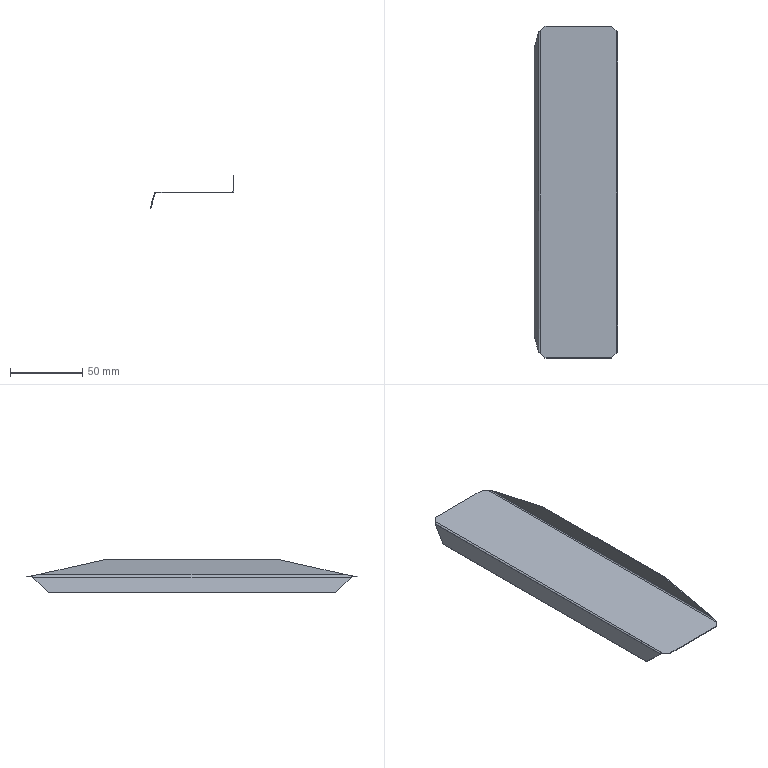Part | SolidWorks | features BaseBody 1 | 1 solid | 28 faces | box 57.977 x 230 x 22.893 mm | volume 8388 mm3 | plane 18 | spline 6 | cylinder 4 | commonest cylinder face diameters 1.5 x2 2.5 x2
STEP:
#1=CARTESIAN_POINT('',(-26.43,-111.57,0.));
#2=VERTEX_POINT('',#1);
#3=CARTESIAN_POINT('',(-26.43,111.57,0.));
#4=VERTEX_POINT('',#3);
#5=CARTESIAN_POINT('',(-26.43,0.,0.));
#6=DIRECTION('',(0.,1.,0.));
#7=VECTOR('',#6,1000.);
#8=LINE('',#5,#7);
#9=EDGE_CURVE('',#2,#4,#8,.T.);
#10=ORIENTED_EDGE('',*,*,#9,.F.);
#11=CARTESIAN_POINT('',(-23.,-115.,0.));
#12=VERTEX_POINT('',#11);
#13=CARTESIAN_POINT('',(-26.43,-111.57,0.));
#14=DIRECTION('',(-0.7071,0.7071,0.));
#15=VECTOR('',#14,1000.);
#16=LINE('',#13,#15);
#17=EDGE_CURVE('',#12,#2,#16,.T.);
#18=ORIENTED_EDGE('',*,*,#17,.F.);
#19=CARTESIAN_POINT('',(23.,-115.,0.));
#20=VERTEX_POINT('',#19);
#21=CARTESIAN_POINT('',(-0.1075,-115.,0.));
#22=DIRECTION('',(-1.,0.,0.));
#23=VECTOR('',#22,1000.);
#24=LINE('',#21,#23);
#25=EDGE_CURVE('',#20,#12,#24,.T.);
#26=ORIENTED_EDGE('',*,*,#25,.F.);
#27=CARTESIAN_POINT('',(26.215,-111.785,0.));
#28=VERTEX_POINT('',#27);
#29=CARTESIAN_POINT('',(23.,-115.,0.));
#30=DIRECTION('',(-0.7071,-0.7071,0.));
#31=VECTOR('',#30,1000.);
#32=LINE('',#29,#31);
#33=EDGE_CURVE('',#28,#20,#32,.T.);
#34=ORIENTED_EDGE('',*,*,#33,.F.);
#35=CARTESIAN_POINT('',(26.215,111.785,0.));
#36=VERTEX_POINT('',#35);
#37=CARTESIAN_POINT('',(26.215,0.,0.));
#38=DIRECTION('',(0.,-1.,0.));
#39=VECTOR('',#38,1000.);
#40=LINE('',#37,#39);
#41=EDGE_CURVE('',#36,#28,#40,.T.);
#42=ORIENTED_EDGE('',*,*,#41,.F.);
#43=CARTESIAN_POINT('',(23.,115.,0.));
#44=VERTEX_POINT('',#43);
#45=CARTESIAN_POINT('',(26.215,111.785,0.));
#46=DIRECTION('',(0.7071,-0.7071,0.));
#47=VECTOR('',#46,1000.);
#48=LINE('',#45,#47);
#49=EDGE_CURVE('',#44,#36,#48,.T.);
#50=ORIENTED_EDGE('',*,*,#49,.F.);
#51=CARTESIAN_POINT('',(-23.,115.,0.));
#52=VERTEX_POINT('',#51);
#53=CARTESIAN_POINT('',(-0.1075,115.,0.));
#54=DIRECTION('',(1.,0.,0.));
#55=VECTOR('',#54,1000.);
#56=LINE('',#53,#55);
#57=EDGE_CURVE('',#52,#44,#56,.T.);
#58=ORIENTED_EDGE('',*,*,#57,.F.);
#59=CARTESIAN_POINT('',(-23.,115.,0.));
#60=DIRECTION('',(0.7071,0.7071,0.));
#61=VECTOR('',#60,1000.);
#62=LINE('',#59,#61);
#63=EDGE_CURVE('',#4,#52,#62,.T.);
#64=ORIENTED_EDGE('',*,*,#63,.F.);
#65=EDGE_LOOP('',(#10,#18,#26,#34,#42,#50,#58,#64));
#66=FACE_OUTER_BOUND('',#65,.T.);
#67=CARTESIAN_POINT('',(26.215,-115.,0.));
#68=DIRECTION('',(0.,0.,-1.));
#69=DIRECTION('',(-1.,0.,0.));
#70=AXIS2_PLACEMENT_3D('',#67,#68,#69);
#71=PLANE('',#70);
#72=ADVANCED_FACE('',(#66),#71,.F.);
#73=CARTESIAN_POINT('',(-23.,115.,-0.5));
#74=VERTEX_POINT('',#73);
#75=CARTESIAN_POINT('',(-23.,115.,-0.25));
#76=DIRECTION('',(0.,0.,-1.));
#77=VECTOR('',#76,1000.);
#78=LINE('',#75,#77);
#79=EDGE_CURVE('',#52,#74,#78,.T.);
#80=ORIENTED_EDGE('',*,*,#79,.T.);
#81=CARTESIAN_POINT('',(-26.43,111.57,-0.5));
#82=VERTEX_POINT('',#81);
#83=CARTESIAN_POINT('',(-24.715,113.285,-0.5));
#84=DIRECTION('',(-0.7071,-0.7071,0.));
#85=VECTOR('',#84,1000.);
#86=LINE('',#83,#85);
#87=EDGE_CURVE('',#74,#82,#86,.T.);
#88=ORIENTED_EDGE('',*,*,#87,.T.);
#89=CARTESIAN_POINT('',(-26.43,111.57,-0.25));
#90=DIRECTION('',(0.,0.,1.));
#91=VECTOR('',#90,1000.);
#92=LINE('',#89,#91);
#93=EDGE_CURVE('',#82,#4,#92,.T.);
#94=ORIENTED_EDGE('',*,*,#93,.T.);
#95=ORIENTED_EDGE('',*,*,#63,.T.);
#96=EDGE_LOOP('',(#80,#88,#94,#95));
#97=FACE_OUTER_BOUND('',#96,.T.);
#98=CARTESIAN_POINT('',(-23.,115.,-0.5));
#99=DIRECTION('',(-0.7071,0.7071,0.));
#100=DIRECTION('',(-0.7071,-0.7071,0.));
#101=AXIS2_PLACEMENT_3D('',#98,#99,#100);
#102=PLANE('',#101);
#103=ADVANCED_FACE('',(#97),#102,.T.);
#104=CARTESIAN_POINT('',(-27.634,110.27,-0.916));
#105=VERTEX_POINT('',#104);
#106=CARTESIAN_POINT('',(-27.634,110.27,-0.916));
#107=CARTESIAN_POINT('',(-27.562,110.487,-0.6549));
#108=CARTESIAN_POINT('',(-27.402,110.703,-0.419));
#109=CARTESIAN_POINT('',(-26.971,111.137,-0.09103));
#110=CARTESIAN_POINT('',(-26.701,111.354,0.));
#111=CARTESIAN_POINT('',(-26.43,111.57,0.));
#112=B_SPLINE_CURVE_WITH_KNOTS('',3,(#106,#107,#108,#109,#110,#111),.UNSPECIFIED.,.F.,.F.,(4,2,4),(0.,0.5,1.),.UNSPECIFIED.);
#113=EDGE_CURVE('',#105,#4,#112,.T.);
#114=ORIENTED_EDGE('',*,*,#113,.F.);
#115=CARTESIAN_POINT('',(-27.634,-110.27,-0.916));
#116=VERTEX_POINT('',#115);
#117=CARTESIAN_POINT('',(-27.634,0.,-0.916));
#118=DIRECTION('',(0.,1.,0.));
#119=VECTOR('',#118,1000.);
#120=LINE('',#117,#119);
#121=EDGE_CURVE('',#116,#105,#120,.T.);
#122=ORIENTED_EDGE('',*,*,#121,.F.);
#123=CARTESIAN_POINT('',(-26.43,-111.57,0.));
#124=CARTESIAN_POINT('',(-26.701,-111.354,0.));
#125=CARTESIAN_POINT('',(-26.971,-111.137,-0.09103));
#126=CARTESIAN_POINT('',(-27.402,-110.703,-0.419));
#127=CARTESIAN_POINT('',(-27.562,-110.487,-0.6549));
#128=CARTESIAN_POINT('',(-27.634,-110.27,-0.916));
#129=B_SPLINE_CURVE_WITH_KNOTS('',3,(#123,#124,#125,#126,#127,#128),.UNSPECIFIED.,.F.,.F.,(4,2,4),(0.,0.5,1.),.UNSPECIFIED.);
#130=EDGE_CURVE('',#2,#116,#129,.T.);
#131=ORIENTED_EDGE('',*,*,#130,.F.);
#132=ORIENTED_EDGE('',*,*,#9,.T.);
#133=EDGE_LOOP('',(#114,#122,#131,#132));
#134=FACE_OUTER_BOUND('',#133,.T.);
#135=CARTESIAN_POINT('',(-26.43,-112.909,-1.25));
#136=DIRECTION('',(0.,1.,0.));
#137=DIRECTION('',(-1.,0.,0.));
#138=AXIS2_PLACEMENT_3D('',#135,#136,#137);
#139=CYLINDRICAL_SURFACE('',#138,1.25);
#140=ADVANCED_FACE('',(#134),#139,.T.);
#141=CARTESIAN_POINT('',(-23.,-115.,-0.5));
#142=VERTEX_POINT('',#141);
#143=CARTESIAN_POINT('',(-23.,-115.,-0.25));
#144=DIRECTION('',(0.,0.,1.));
#145=VECTOR('',#144,1000.);
#146=LINE('',#143,#145);
#147=EDGE_CURVE('',#142,#12,#146,.T.);
#148=ORIENTED_EDGE('',*,*,#147,.T.);
#149=ORIENTED_EDGE('',*,*,#17,.T.);
#150=CARTESIAN_POINT('',(-26.43,-111.57,-0.5));
#151=VERTEX_POINT('',#150);
#152=CARTESIAN_POINT('',(-26.43,-111.57,-0.25));
#153=DIRECTION('',(0.,0.,-1.));
#154=VECTOR('',#153,1000.);
#155=LINE('',#152,#154);
#156=EDGE_CURVE('',#2,#151,#155,.T.);
#157=ORIENTED_EDGE('',*,*,#156,.T.);
#158=CARTESIAN_POINT('',(-24.715,-113.285,-0.5));
#159=DIRECTION('',(0.7071,-0.7071,0.));
#160=VECTOR('',#159,1000.);
#161=LINE('',#158,#160);
#162=EDGE_CURVE('',#151,#142,#161,.T.);
#163=ORIENTED_EDGE('',*,*,#162,.T.);
#164=EDGE_LOOP('',(#148,#149,#157,#163));
#165=FACE_OUTER_BOUND('',#164,.T.);
#166=CARTESIAN_POINT('',(-26.43,-111.57,-0.5));
#167=DIRECTION('',(-0.7071,-0.7071,0.));
#168=DIRECTION('',(0.7071,-0.7071,0.));
#169=AXIS2_PLACEMENT_3D('',#166,#167,#168);
#170=PLANE('',#169);
#171=ADVANCED_FACE('',(#165),#170,.T.);
#172=CARTESIAN_POINT('',(23.,-115.,-0.5));
#173=VERTEX_POINT('',#172);
#174=CARTESIAN_POINT('',(0.,-115.,-0.5));
#175=DIRECTION('',(1.,0.,0.));
#176=VECTOR('',#175,1000.);
#177=LINE('',#174,#176);
#178=EDGE_CURVE('',#142,#173,#177,.T.);
#179=ORIENTED_EDGE('',*,*,#178,.T.);
#180=CARTESIAN_POINT('',(23.,-115.,-0.25));
#181=DIRECTION('',(0.,0.,1.));
#182=VECTOR('',#181,1000.);
#183=LINE('',#180,#182);
#184=EDGE_CURVE('',#173,#20,#183,.T.);
#185=ORIENTED_EDGE('',*,*,#184,.T.);
#186=ORIENTED_EDGE('',*,*,#25,.T.);
#187=ORIENTED_EDGE('',*,*,#147,.F.);
#188=EDGE_LOOP('',(#179,#185,#186,#187));
#189=FACE_OUTER_BOUND('',#188,.T.);
#190=CARTESIAN_POINT('',(-23.,-115.,-0.5));
#191=DIRECTION('',(0.,-1.,0.));
#192=DIRECTION('',(1.,0.,0.));
#193=AXIS2_PLACEMENT_3D('',#190,#191,#192);
#194=PLANE('',#193);
#195=ADVANCED_FACE('',(#189),#194,.T.);
#196=ORIENTED_EDGE('',*,*,#33,.T.);
#197=ORIENTED_EDGE('',*,*,#184,.F.);
#198=CARTESIAN_POINT('',(26.215,-111.785,-0.5));
#199=VERTEX_POINT('',#198);
#200=CARTESIAN_POINT('',(24.607,-113.393,-0.5));
#201=DIRECTION('',(0.7071,0.7071,0.));
#202=VECTOR('',#201,1000.);
#203=LINE('',#200,#202);
#204=EDGE_CURVE('',#173,#199,#203,.T.);
#205=ORIENTED_EDGE('',*,*,#204,.T.);
#206=CARTESIAN_POINT('',(26.215,-111.785,-0.25));
#207=DIRECTION('',(0.,0.,1.));
#208=VECTOR('',#207,1000.);
#209=LINE('',#206,#208);
#210=EDGE_CURVE('',#199,#28,#209,.T.);
#211=ORIENTED_EDGE('',*,*,#210,.T.);
#212=EDGE_LOOP('',(#196,#197,#205,#211));
#213=FACE_OUTER_BOUND('',#212,.T.);
#214=CARTESIAN_POINT('',(23.,-115.,-0.5));
#215=DIRECTION('',(0.7071,-0.7071,0.));
#216=DIRECTION('',(0.7071,0.7071,0.));
#217=AXIS2_PLACEMENT_3D('',#214,#215,#216);
#218=PLANE('',#217);
#219=ADVANCED_FACE('',(#213),#218,.T.);
#220=ORIENTED_EDGE('',*,*,#41,.T.);
#221=CARTESIAN_POINT('',(26.745,-111.,0.2197));
#222=VERTEX_POINT('',#221);
#223=CARTESIAN_POINT('',(26.215,-111.785,0.));
#224=CARTESIAN_POINT('',(26.411,-111.523,0.000000004));
#225=CARTESIAN_POINT('',(26.606,-111.262,0.08077));
#226=CARTESIAN_POINT('',(26.745,-111.,0.2197));
#227=B_SPLINE_CURVE_WITH_KNOTS('',3,(#223,#224,#225,#226),.UNSPECIFIED.,.F.,.F.,(4,4),(0.,0.0009817),.UNSPECIFIED.);
#228=EDGE_CURVE('',#28,#222,#227,.T.);
#229=ORIENTED_EDGE('',*,*,#228,.T.);
#230=CARTESIAN_POINT('',(26.965,-107.517,0.75));
#231=VERTEX_POINT('',#230);
#232=CARTESIAN_POINT('',(26.745,-111.,0.2197));
#233=CARTESIAN_POINT('',(26.884,-109.839,0.3585));
#234=CARTESIAN_POINT('',(26.965,-108.678,0.5536));
#235=CARTESIAN_POINT('',(26.965,-107.517,0.75));
#236=B_SPLINE_CURVE_WITH_KNOTS('',3,(#232,#233,#234,#235),.UNSPECIFIED.,.F.,.F.,(4,4),(0.,0.003533),.UNSPECIFIED.);
#237=EDGE_CURVE('',#222,#231,#236,.T.);
#238=ORIENTED_EDGE('',*,*,#237,.T.);
#239=CARTESIAN_POINT('',(26.965,107.517,0.75));
#240=VERTEX_POINT('',#239);
#241=CARTESIAN_POINT('',(26.965,0.,0.75));
#242=DIRECTION('',(0.,1.,0.));
#243=VECTOR('',#242,1000.);
#244=LINE('',#241,#243);
#245=EDGE_CURVE('',#231,#240,#244,.T.);
#246=ORIENTED_EDGE('',*,*,#245,.T.);
#247=CARTESIAN_POINT('',(26.745,111.,0.2197));
#248=VERTEX_POINT('',#247);
#249=CARTESIAN_POINT('',(26.965,107.517,0.75));
#250=CARTESIAN_POINT('',(26.965,108.678,0.5536));
#251=CARTESIAN_POINT('',(26.884,109.839,0.3585));
#252=CARTESIAN_POINT('',(26.745,111.,0.2197));
#253=B_SPLINE_CURVE_WITH_KNOTS('',3,(#249,#250,#251,#252),.UNSPECIFIED.,.F.,.F.,(4,4),(0.,0.003533),.UNSPECIFIED.);
#254=EDGE_CURVE('',#240,#248,#253,.T.);
#255=ORIENTED_EDGE('',*,*,#254,.T.);
#256=CARTESIAN_POINT('',(26.745,111.,0.2197));
#257=CARTESIAN_POINT('',(26.606,111.262,0.08073));
#258=CARTESIAN_POINT('',(26.411,111.523,0.000000004));
#259=CARTESIAN_POINT('',(26.215,111.785,0.));
#260=B_SPLINE_CURVE_WITH_KNOTS('',3,(#256,#257,#258,#259),.UNSPECIFIED.,.F.,.F.,(4,4),(0.,0.0009806),.UNSPECIFIED.);
#261=EDGE_CURVE('',#248,#36,#260,.T.);
#262=ORIENTED_EDGE('',*,*,#261,.T.);
#263=EDGE_LOOP('',(#220,#229,#238,#246,#255,#262));
#264=FACE_OUTER_BOUND('',#263,.T.);
#265=CARTESIAN_POINT('',(26.215,113.127,0.75));
#266=DIRECTION('',(0.,-1.,0.));
#267=DIRECTION('',(0.,0.,-1.));
#268=AXIS2_PLACEMENT_3D('',#265,#266,#267);
#269=CYLINDRICAL_SURFACE('',#268,0.75);
#270=ADVANCED_FACE('',(#264),#269,.F.);
#271=CARTESIAN_POINT('',(26.215,111.785,-0.5));
#272=VERTEX_POINT('',#271);
#273=CARTESIAN_POINT('',(23.,115.,-0.5));
#274=VERTEX_POINT('',#273);
#275=CARTESIAN_POINT('',(24.607,113.393,-0.5));
#276=DIRECTION('',(-0.7071,0.7071,0.));
#277=VECTOR('',#276,1000.);
#278=LINE('',#275,#277);
#279=EDGE_CURVE('',#272,#274,#278,.T.);
#280=ORIENTED_EDGE('',*,*,#279,.T.);
#281=CARTESIAN_POINT('',(23.,115.,-0.25));
#282=DIRECTION('',(0.,0.,1.));
#283=VECTOR('',#282,1000.);
#284=LINE('',#281,#283);
#285=EDGE_CURVE('',#274,#44,#284,.T.);
#286=ORIENTED_EDGE('',*,*,#285,.T.);
#287=ORIENTED_EDGE('',*,*,#49,.T.);
#288=CARTESIAN_POINT('',(26.215,111.785,-0.25));
#289=DIRECTION('',(0.,0.,-1.));
#290=VECTOR('',#289,1000.);
#291=LINE('',#288,#290);
#292=EDGE_CURVE('',#36,#272,#291,.T.);
#293=ORIENTED_EDGE('',*,*,#292,.T.);
#294=EDGE_LOOP('',(#280,#286,#287,#293));
#295=FACE_OUTER_BOUND('',#294,.T.);
#296=CARTESIAN_POINT('',(26.215,111.785,-0.5));
#297=DIRECTION('',(0.7071,0.7071,0.));
#298=DIRECTION('',(-0.7071,0.7071,0.));
#299=AXIS2_PLACEMENT_3D('',#296,#297,#298);
#300=PLANE('',#299);
#301=ADVANCED_FACE('',(#295),#300,.T.);
#302=CARTESIAN_POINT('',(0.,115.,-0.5));
#303=DIRECTION('',(-1.,0.,0.));
#304=VECTOR('',#303,1000.);
#305=LINE('',#302,#304);
#306=EDGE_CURVE('',#274,#74,#305,.T.);
#307=ORIENTED_EDGE('',*,*,#306,.T.);
#308=ORIENTED_EDGE('',*,*,#79,.F.);
#309=ORIENTED_EDGE('',*,*,#57,.T.);
#310=ORIENTED_EDGE('',*,*,#285,.F.);
#311=EDGE_LOOP('',(#307,#308,#309,#310));
#312=FACE_OUTER_BOUND('',#311,.T.);
#313=CARTESIAN_POINT('',(23.,115.,-0.5));
#314=DIRECTION('',(0.,1.,0.));
#315=DIRECTION('',(-1.,0.,0.));
#316=AXIS2_PLACEMENT_3D('',#313,#314,#315);
#317=PLANE('',#316);
#318=ADVANCED_FACE('',(#312),#317,.T.);
#319=ORIENTED_EDGE('',*,*,#178,.F.);
#320=ORIENTED_EDGE('',*,*,#162,.F.);
#321=CARTESIAN_POINT('',(-26.43,0.,-0.5));
#322=DIRECTION('',(0.,1.,0.));
#323=VECTOR('',#322,1000.);
#324=LINE('',#321,#323);
#325=EDGE_CURVE('',#151,#82,#324,.T.);
#326=ORIENTED_EDGE('',*,*,#325,.T.);
#327=ORIENTED_EDGE('',*,*,#87,.F.);
#328=ORIENTED_EDGE('',*,*,#306,.F.);
#329=ORIENTED_EDGE('',*,*,#279,.F.);
#330=CARTESIAN_POINT('',(26.215,0.,-0.5));
#331=DIRECTION('',(0.,-1.,0.));
#332=VECTOR('',#331,1000.);
#333=LINE('',#330,#332);
#334=EDGE_CURVE('',#272,#199,#333,.T.);
#335=ORIENTED_EDGE('',*,*,#334,.T.);
#336=ORIENTED_EDGE('',*,*,#204,.F.);
#337=EDGE_LOOP('',(#319,#320,#326,#327,#328,#329,#335,#336));
#338=FACE_OUTER_BOUND('',#337,.T.);
#339=CARTESIAN_POINT('',(26.215,-115.,-0.5));
#340=DIRECTION('',(0.,0.,-1.));
#341=DIRECTION('',(-1.,0.,0.));
#342=AXIS2_PLACEMENT_3D('',#339,#340,#341);
#343=PLANE('',#342);
#344=ADVANCED_FACE('',(#338),#343,.T.);
#345=ORIENTED_EDGE('',*,*,#113,.T.);
#346=ORIENTED_EDGE('',*,*,#93,.F.);
#347=CARTESIAN_POINT('',(-27.152,110.27,-1.05));
#348=VERTEX_POINT('',#347);
#349=CARTESIAN_POINT('',(-27.152,110.27,-1.05));
#350=CARTESIAN_POINT('',(-27.109,110.487,-0.8929));
#351=CARTESIAN_POINT('',(-27.013,110.703,-0.7514));
#352=CARTESIAN_POINT('',(-26.754,111.137,-0.5546));
#353=CARTESIAN_POINT('',(-26.592,111.354,-0.5));
#354=CARTESIAN_POINT('',(-26.43,111.57,-0.5));
#355=B_SPLINE_CURVE_WITH_KNOTS('',3,(#349,#350,#351,#352,#353,#354),.UNSPECIFIED.,.F.,.F.,(4,2,4),(0.,0.5,1.),.UNSPECIFIED.);
#356=EDGE_CURVE('',#348,#82,#355,.T.);
#357=ORIENTED_EDGE('',*,*,#356,.F.);
#358=CARTESIAN_POINT('',(-27.393,110.27,-0.9828));
#359=DIRECTION('',(0.9636,0.,-0.2672));
#360=VECTOR('',#359,1000.);
#361=LINE('',#358,#360);
#362=EDGE_CURVE('',#105,#348,#361,.T.);
#363=ORIENTED_EDGE('',*,*,#362,.F.);
#364=EDGE_LOOP('',(#345,#346,#357,#363));
#365=FACE_OUTER_BOUND('',#364,.T.);
#366=CARTESIAN_POINT('',(-27.639,110.27,-0.9146));
#367=CARTESIAN_POINT('',(-27.603,110.378,-0.7836));
#368=CARTESIAN_POINT('',(-27.545,110.487,-0.6585));
#369=CARTESIAN_POINT('',(-27.392,110.703,-0.4334));
#370=CARTESIAN_POINT('',(-27.298,110.812,-0.3333));
#371=CARTESIAN_POINT('',(-27.081,111.029,-0.1687));
#372=CARTESIAN_POINT('',(-26.959,111.137,-0.1042));
#373=CARTESIAN_POINT('',(-26.702,111.354,-0.01729));
#374=CARTESIAN_POINT('',(-26.566,111.462,0.005));
#375=CARTESIAN_POINT('',(-26.43,111.57,0.005));
#376=CARTESIAN_POINT('',(-27.634,110.27,-0.916));
#377=CARTESIAN_POINT('',(-27.598,110.378,-0.7854));
#378=CARTESIAN_POINT('',(-27.54,110.487,-0.6609));
#379=CARTESIAN_POINT('',(-27.388,110.703,-0.4366));
#380=CARTESIAN_POINT('',(-27.294,110.812,-0.337));
#381=CARTESIAN_POINT('',(-27.078,111.029,-0.173));
#382=CARTESIAN_POINT('',(-26.957,111.137,-0.1087));
#383=CARTESIAN_POINT('',(-26.701,111.354,-0.02221));
#384=CARTESIAN_POINT('',(-26.565,111.462,0.));
#385=CARTESIAN_POINT('',(-26.43,111.57,0.));
#386=CARTESIAN_POINT('',(-27.152,110.27,-1.05));
#387=CARTESIAN_POINT('',(-27.131,110.378,-0.9713));
#388=CARTESIAN_POINT('',(-27.096,110.487,-0.8965));
#389=CARTESIAN_POINT('',(-27.005,110.703,-0.762));
#390=CARTESIAN_POINT('',(-26.948,110.812,-0.7022));
#391=CARTESIAN_POINT('',(-26.819,111.029,-0.6038));
#392=CARTESIAN_POINT('',(-26.746,111.137,-0.5652));
#393=CARTESIAN_POINT('',(-26.592,111.354,-0.5133));
#394=CARTESIAN_POINT('',(-26.511,111.462,-0.5));
#395=CARTESIAN_POINT('',(-26.43,111.57,-0.5));
#396=CARTESIAN_POINT('',(-27.148,110.27,-1.051));
#397=CARTESIAN_POINT('',(-27.126,110.378,-0.9731));
#398=CARTESIAN_POINT('',(-27.092,110.487,-0.8989));
#399=CARTESIAN_POINT('',(-27.001,110.703,-0.7653));
#400=CARTESIAN_POINT('',(-26.945,110.812,-0.7059));
#401=CARTESIAN_POINT('',(-26.816,111.029,-0.6082));
#402=CARTESIAN_POINT('',(-26.744,111.137,-0.5698));
#403=CARTESIAN_POINT('',(-26.591,111.354,-0.5183));
#404=CARTESIAN_POINT('',(-26.51,111.462,-0.505));
#405=CARTESIAN_POINT('',(-26.43,111.57,-0.505));
#406=B_SPLINE_SURFACE_WITH_KNOTS('',1,3,((#366,#367,#368,#369,#370,#371,#372,#373,#374,#375),(#376,#377,#378,#379,#380,#381,#382,#383,#384,#385),(#386,#387,#388,#389,#390,#391,#392,#393,#394,#395),(#396,#397,#398,#399,#400,#401,#402,#403,#404,#405)),.UNSPECIFIED.,.F.,.F.,.F.,(2,1,1,2),(4,2,2,2,4),(-0.01,0.,1.,1.01),(0.,0.25,0.5,0.75,1.),.UNSPECIFIED.);
#407=ADVANCED_FACE('',(#365),#406,.F.);
#408=CARTESIAN_POINT('',(-30.512,99.5,-11.294));
#409=VERTEX_POINT('',#408);
#410=CARTESIAN_POINT('',(-27.634,110.27,-0.916));
#411=DIRECTION('',(0.189,0.7071,0.6814));
#412=VECTOR('',#411,1000.);
#413=LINE('',#410,#412);
#414=EDGE_CURVE('',#409,#105,#413,.T.);
#415=ORIENTED_EDGE('',*,*,#414,.F.);
#416=CARTESIAN_POINT('',(-30.512,-99.5,-11.294));
#417=VERTEX_POINT('',#416);
#418=CARTESIAN_POINT('',(-30.512,0.,-11.294));
#419=DIRECTION('',(0.,1.,0.));
#420=VECTOR('',#419,1000.);
#421=LINE('',#418,#420);
#422=EDGE_CURVE('',#417,#409,#421,.T.);
#423=ORIENTED_EDGE('',*,*,#422,.F.);
#424=CARTESIAN_POINT('',(-30.512,-99.5,-11.294));
#425=DIRECTION('',(-0.189,0.7071,-0.6814));
#426=VECTOR('',#425,1000.);
#427=LINE('',#424,#426);
#428=EDGE_CURVE('',#116,#417,#427,.T.);
#429=ORIENTED_EDGE('',*,*,#428,.F.);
#430=ORIENTED_EDGE('',*,*,#121,.T.);
#431=EDGE_LOOP('',(#415,#423,#429,#430));
#432=FACE_OUTER_BOUND('',#431,.T.);
#433=CARTESIAN_POINT('',(-27.634,-111.593,-0.916));
#434=DIRECTION('',(0.9636,0.,-0.2672));
#435=DIRECTION('',(-0.2672,0.,-0.9636));
#436=AXIS2_PLACEMENT_3D('',#433,#434,#435);
#437=PLANE('',#436);
#438=ADVANCED_FACE('',(#432),#437,.F.);
#439=CARTESIAN_POINT('',(-27.152,-110.27,-1.05));
#440=VERTEX_POINT('',#439);
#441=CARTESIAN_POINT('',(-27.393,-110.27,-0.9828));
#442=DIRECTION('',(-0.9636,0.,0.2672));
#443=VECTOR('',#442,1000.);
#444=LINE('',#441,#443);
#445=EDGE_CURVE('',#440,#116,#444,.T.);
#446=ORIENTED_EDGE('',*,*,#445,.F.);
#447=CARTESIAN_POINT('',(-26.43,-111.57,-0.5));
#448=CARTESIAN_POINT('',(-26.592,-111.354,-0.5));
#449=CARTESIAN_POINT('',(-26.754,-111.137,-0.5546));
#450=CARTESIAN_POINT('',(-27.013,-110.703,-0.7514));
#451=CARTESIAN_POINT('',(-27.109,-110.487,-0.8929));
#452=CARTESIAN_POINT('',(-27.152,-110.27,-1.05));
#453=B_SPLINE_CURVE_WITH_KNOTS('',3,(#447,#448,#449,#450,#451,#452),.UNSPECIFIED.,.F.,.F.,(4,2,4),(0.,0.5,1.),.UNSPECIFIED.);
#454=EDGE_CURVE('',#151,#440,#453,.T.);
#455=ORIENTED_EDGE('',*,*,#454,.F.);
#456=ORIENTED_EDGE('',*,*,#156,.F.);
#457=ORIENTED_EDGE('',*,*,#130,.T.);
#458=EDGE_LOOP('',(#446,#455,#456,#457));
#459=FACE_OUTER_BOUND('',#458,.T.);
#460=CARTESIAN_POINT('',(-26.43,-111.57,0.005));
#461=CARTESIAN_POINT('',(-26.566,-111.462,0.005));
#462=CARTESIAN_POINT('',(-26.702,-111.354,-0.01729));
#463=CARTESIAN_POINT('',(-26.959,-111.137,-0.1042));
#464=CARTESIAN_POINT('',(-27.081,-111.029,-0.1687));
#465=CARTESIAN_POINT('',(-27.298,-110.812,-0.3333));
#466=CARTESIAN_POINT('',(-27.392,-110.703,-0.4334));
#467=CARTESIAN_POINT('',(-27.545,-110.487,-0.6585));
#468=CARTESIAN_POINT('',(-27.603,-110.378,-0.7836));
#469=CARTESIAN_POINT('',(-27.639,-110.27,-0.9146));
#470=CARTESIAN_POINT('',(-26.43,-111.57,0.));
#471=CARTESIAN_POINT('',(-26.565,-111.462,0.));
#472=CARTESIAN_POINT('',(-26.701,-111.354,-0.02221));
#473=CARTESIAN_POINT('',(-26.957,-111.137,-0.1087));
#474=CARTESIAN_POINT('',(-27.078,-111.029,-0.173));
#475=CARTESIAN_POINT('',(-27.294,-110.812,-0.337));
#476=CARTESIAN_POINT('',(-27.388,-110.703,-0.4366));
#477=CARTESIAN_POINT('',(-27.54,-110.487,-0.6609));
#478=CARTESIAN_POINT('',(-27.598,-110.378,-0.7854));
#479=CARTESIAN_POINT('',(-27.634,-110.27,-0.916));
#480=CARTESIAN_POINT('',(-26.43,-111.57,-0.5));
#481=CARTESIAN_POINT('',(-26.511,-111.462,-0.5));
#482=CARTESIAN_POINT('',(-26.592,-111.354,-0.5133));
#483=CARTESIAN_POINT('',(-26.746,-111.137,-0.5652));
#484=CARTESIAN_POINT('',(-26.819,-111.029,-0.6038));
#485=CARTESIAN_POINT('',(-26.948,-110.812,-0.7022));
#486=CARTESIAN_POINT('',(-27.005,-110.703,-0.762));
#487=CARTESIAN_POINT('',(-27.096,-110.487,-0.8965));
#488=CARTESIAN_POINT('',(-27.131,-110.378,-0.9713));
#489=CARTESIAN_POINT('',(-27.152,-110.27,-1.05));
#490=CARTESIAN_POINT('',(-26.43,-111.57,-0.505));
#491=CARTESIAN_POINT('',(-26.51,-111.462,-0.505));
#492=CARTESIAN_POINT('',(-26.591,-111.354,-0.5183));
#493=CARTESIAN_POINT('',(-26.744,-111.137,-0.5698));
#494=CARTESIAN_POINT('',(-26.816,-111.029,-0.6082));
#495=CARTESIAN_POINT('',(-26.945,-110.812,-0.7059));
#496=CARTESIAN_POINT('',(-27.001,-110.703,-0.7653));
#497=CARTESIAN_POINT('',(-27.092,-110.487,-0.8989));
#498=CARTESIAN_POINT('',(-27.126,-110.378,-0.9731));
#499=CARTESIAN_POINT('',(-27.148,-110.27,-1.051));
#500=B_SPLINE_SURFACE_WITH_KNOTS('',1,3,((#460,#461,#462,#463,#464,#465,#466,#467,#468,#469),(#470,#471,#472,#473,#474,#475,#476,#477,#478,#479),(#480,#481,#482,#483,#484,#485,#486,#487,#488,#489),(#490,#491,#492,#493,#494,#495,#496,#497,#498,#499)),.UNSPECIFIED.,.F.,.F.,.F.,(2,1,1,2),(4,2,2,2,4),(-0.01,0.,1.,1.01),(0.,0.25,0.5,0.75,1.),.UNSPECIFIED.);
#501=ADVANCED_FACE('',(#459),#500,.F.);
#502=CARTESIAN_POINT('',(27.098,-111.,-0.1339));
#503=VERTEX_POINT('',#502);
#504=CARTESIAN_POINT('',(26.215,-111.785,-0.5));
#505=CARTESIAN_POINT('',(26.379,-111.654,-0.5));
#506=CARTESIAN_POINT('',(26.542,-111.523,-0.4674));
#507=CARTESIAN_POINT('',(26.845,-111.261,-0.3416));
#508=CARTESIAN_POINT('',(26.982,-111.131,-0.2501));
#509=CARTESIAN_POINT('',(27.098,-111.,-0.1339));
#510=B_SPLINE_CURVE_WITH_KNOTS('',3,(#504,#505,#506,#507,#508,#509),.UNSPECIFIED.,.F.,.F.,(4,2,4),(0.,0.0006291,0.001258),.UNSPECIFIED.);
#511=EDGE_CURVE('',#199,#503,#510,.T.);
#512=ORIENTED_EDGE('',*,*,#511,.T.);
#513=CARTESIAN_POINT('',(26.922,-111.,0.04289));
#514=DIRECTION('',(-0.7071,0.,0.7071));
#515=VECTOR('',#514,1000.);
#516=LINE('',#513,#515);
#517=EDGE_CURVE('',#503,#222,#516,.T.);
#518=ORIENTED_EDGE('',*,*,#517,.T.);
#519=ORIENTED_EDGE('',*,*,#228,.F.);
#520=ORIENTED_EDGE('',*,*,#210,.F.);
#521=EDGE_LOOP('',(#512,#518,#519,#520));
#522=FACE_OUTER_BOUND('',#521,.T.);
#523=CARTESIAN_POINT('',(27.102,-111.,-0.1375));
#524=CARTESIAN_POINT('',(26.986,-111.131,-0.2536));
#525=CARTESIAN_POINT('',(26.847,-111.262,-0.3466));
#526=CARTESIAN_POINT('',(26.543,-111.524,-0.4724));
#527=CARTESIAN_POINT('',(26.379,-111.654,-0.505));
#528=CARTESIAN_POINT('',(26.215,-111.785,-0.505));
#529=CARTESIAN_POINT('',(27.098,-111.,-0.1339));
#530=CARTESIAN_POINT('',(26.983,-111.131,-0.2496));
#531=CARTESIAN_POINT('',(26.844,-111.262,-0.3422));
#532=CARTESIAN_POINT('',(26.542,-111.524,-0.4675));
#533=CARTESIAN_POINT('',(26.378,-111.654,-0.5));
#534=CARTESIAN_POINT('',(26.215,-111.785,-0.5));
#535=CARTESIAN_POINT('',(26.745,-111.,0.2197));
#536=CARTESIAN_POINT('',(26.676,-111.131,0.1502));
#537=CARTESIAN_POINT('',(26.592,-111.262,0.09466));
#538=CARTESIAN_POINT('',(26.411,-111.524,0.01952));
#539=CARTESIAN_POINT('',(26.313,-111.654,0.));
#540=CARTESIAN_POINT('',(26.215,-111.785,0.));
#541=CARTESIAN_POINT('',(26.741,-111.,0.2232));
#542=CARTESIAN_POINT('',(26.672,-111.131,0.1542));
#543=CARTESIAN_POINT('',(26.59,-111.262,0.09903));
#544=CARTESIAN_POINT('',(26.41,-111.524,0.02439));
#545=CARTESIAN_POINT('',(26.312,-111.654,0.005));
#546=CARTESIAN_POINT('',(26.215,-111.785,0.005));
#547=B_SPLINE_SURFACE_WITH_KNOTS('',1,3,((#523,#524,#525,#526,#527,#528),(#529,#530,#531,#532,#533,#534),(#535,#536,#537,#538,#539,#540),(#541,#542,#543,#544,#545,#546)),.UNSPECIFIED.,.F.,.F.,.F.,(2,1,1,2),(4,2,4),(-0.0101,0.,1.,1.01),(0.,0.5,1.),.UNSPECIFIED.);
#548=ADVANCED_FACE('',(#522),#547,.T.);
#549=CARTESIAN_POINT('',(27.098,111.,-0.1339));
#550=VERTEX_POINT('',#549);
#551=CARTESIAN_POINT('',(26.922,111.,0.04289));
#552=DIRECTION('',(0.7071,0.,-0.7071));
#553=VECTOR('',#552,1000.);
#554=LINE('',#551,#553);
#555=EDGE_CURVE('',#248,#550,#554,.T.);
#556=ORIENTED_EDGE('',*,*,#555,.T.);
#557=CARTESIAN_POINT('',(27.098,111.,-0.1339));
#558=CARTESIAN_POINT('',(26.982,111.131,-0.2501));
#559=CARTESIAN_POINT('',(26.844,111.262,-0.3425));
#560=CARTESIAN_POINT('',(26.541,111.525,-0.4679));
#561=CARTESIAN_POINT('',(26.379,111.654,-0.5));
#562=CARTESIAN_POINT('',(26.215,111.785,-0.5));
#563=B_SPLINE_CURVE_WITH_KNOTS('',3,(#557,#558,#559,#560,#561,#562),.UNSPECIFIED.,.F.,.F.,(4,2,4),(0.,0.0006291,0.001258),.UNSPECIFIED.);
#564=EDGE_CURVE('',#550,#272,#563,.T.);
#565=ORIENTED_EDGE('',*,*,#564,.T.);
#566=ORIENTED_EDGE('',*,*,#292,.F.);
#567=ORIENTED_EDGE('',*,*,#261,.F.);
#568=EDGE_LOOP('',(#556,#565,#566,#567));
#569=FACE_OUTER_BOUND('',#568,.T.);
#570=CARTESIAN_POINT('',(26.215,111.785,-0.505));
#571=CARTESIAN_POINT('',(26.379,111.654,-0.505));
#572=CARTESIAN_POINT('',(26.543,111.524,-0.4724));
#573=CARTESIAN_POINT('',(26.847,111.262,-0.3466));
#574=CARTESIAN_POINT('',(26.986,111.131,-0.2536));
#575=CARTESIAN_POINT('',(27.102,111.,-0.1375));
#576=CARTESIAN_POINT('',(27.104,110.997,-0.1351));
#577=CARTESIAN_POINT('',(27.107,110.995,-0.1328));
#578=CARTESIAN_POINT('',(27.109,110.992,-0.1305));
#579=CARTESIAN_POINT('',(26.215,111.785,-0.5));
#580=CARTESIAN_POINT('',(26.378,111.654,-0.5));
#581=CARTESIAN_POINT('',(26.542,111.524,-0.4675));
#582=CARTESIAN_POINT('',(26.844,111.262,-0.3422));
#583=CARTESIAN_POINT('',(26.983,111.131,-0.2496));
#584=CARTESIAN_POINT('',(27.098,111.,-0.1339));
#585=CARTESIAN_POINT('',(27.101,110.997,-0.1316));
#586=CARTESIAN_POINT('',(27.103,110.995,-0.1293));
#587=CARTESIAN_POINT('',(27.105,110.992,-0.1269));
#588=CARTESIAN_POINT('',(26.215,111.785,0.));
#589=CARTESIAN_POINT('',(26.313,111.654,0.));
#590=CARTESIAN_POINT('',(26.411,111.524,0.01952));
#591=CARTESIAN_POINT('',(26.592,111.262,0.09466));
#592=CARTESIAN_POINT('',(26.676,111.131,0.1502));
#593=CARTESIAN_POINT('',(26.745,111.,0.2197));
#594=CARTESIAN_POINT('',(26.746,110.997,0.2211));
#595=CARTESIAN_POINT('',(26.748,110.995,0.2224));
#596=CARTESIAN_POINT('',(26.749,110.992,0.2238));
#597=CARTESIAN_POINT('',(26.215,111.785,0.005));
#598=CARTESIAN_POINT('',(26.312,111.654,0.005));
#599=CARTESIAN_POINT('',(26.41,111.524,0.02439));
#600=CARTESIAN_POINT('',(26.59,111.262,0.09903));
#601=CARTESIAN_POINT('',(26.672,111.131,0.1542));
#602=CARTESIAN_POINT('',(26.741,111.,0.2232));
#603=CARTESIAN_POINT('',(26.743,110.997,0.2246));
#604=CARTESIAN_POINT('',(26.744,110.995,0.226));
#605=CARTESIAN_POINT('',(26.746,110.992,0.2273));
#606=B_SPLINE_SURFACE_WITH_KNOTS('',1,3,((#570,#571,#572,#573,#574,#575,#576,#577,#578),(#579,#580,#581,#582,#583,#584,#585,#586,#587),(#588,#589,#590,#591,#592,#593,#594,#595,#596),(#597,#598,#599,#600,#601,#602,#603,#604,#605)),.UNSPECIFIED.,.F.,.F.,.F.,(2,1,1,2),(4,2,3,4),(-0.0101,0.,1.,1.01),(0.,0.5,1.,1.01),.UNSPECIFIED.);
#607=ADVANCED_FACE('',(#569),#606,.T.);
#608=CARTESIAN_POINT('',(27.465,107.517,0.75));
#609=VERTEX_POINT('',#608);
#610=CARTESIAN_POINT('',(27.215,107.517,0.75));
#611=DIRECTION('',(-1.,0.,0.));
#612=VECTOR('',#611,1000.);
#613=LINE('',#610,#612);
#614=EDGE_CURVE('',#609,#240,#613,.T.);
#615=ORIENTED_EDGE('',*,*,#614,.F.);
#616=CARTESIAN_POINT('',(27.465,107.517,0.75));
#617=CARTESIAN_POINT('',(27.465,108.098,0.5863));
#618=CARTESIAN_POINT('',(27.432,108.678,0.4228));
#619=CARTESIAN_POINT('',(27.307,109.839,0.1204));
#620=CARTESIAN_POINT('',(27.214,110.419,-0.01813));
#621=CARTESIAN_POINT('',(27.098,111.,-0.1339));
#622=B_SPLINE_CURVE_WITH_KNOTS('',3,(#616,#617,#618,#619,#620,#621),.UNSPECIFIED.,.F.,.F.,(4,2,4),(0.,0.001809,0.003619),.UNSPECIFIED.);
#623=EDGE_CURVE('',#609,#550,#622,.T.);
#624=ORIENTED_EDGE('',*,*,#623,.T.);
#625=ORIENTED_EDGE('',*,*,#555,.F.);
#626=ORIENTED_EDGE('',*,*,#254,.F.);
#627=EDGE_LOOP('',(#615,#624,#625,#626));
#628=FACE_OUTER_BOUND('',#627,.T.);
#629=CARTESIAN_POINT('',(27.102,111.,-0.1375));
#630=CARTESIAN_POINT('',(27.218,110.419,-0.02129));
#631=CARTESIAN_POINT('',(27.311,109.839,0.1179));
#632=CARTESIAN_POINT('',(27.437,108.678,0.4215));
#633=CARTESIAN_POINT('',(27.47,108.097,0.5857));
#634=CARTESIAN_POINT('',(27.47,107.517,0.75));
#635=CARTESIAN_POINT('',(27.098,111.,-0.1339));
#636=CARTESIAN_POINT('',(27.214,110.419,-0.01818));
#637=CARTESIAN_POINT('',(27.307,109.839,0.1205));
#638=CARTESIAN_POINT('',(27.432,108.678,0.4228));
#639=CARTESIAN_POINT('',(27.465,108.097,0.5864));
#640=CARTESIAN_POINT('',(27.465,107.517,0.75));
#641=CARTESIAN_POINT('',(26.745,111.,0.2197));
#642=CARTESIAN_POINT('',(26.814,110.419,0.2891));
#643=CARTESIAN_POINT('',(26.87,109.839,0.3723));
#644=CARTESIAN_POINT('',(26.945,108.678,0.5537));
#645=CARTESIAN_POINT('',(26.965,108.097,0.6518));
#646=CARTESIAN_POINT('',(26.965,107.517,0.75));
#647=CARTESIAN_POINT('',(26.741,111.,0.2232));
#648=CARTESIAN_POINT('',(26.81,110.419,0.2922));
#649=CARTESIAN_POINT('',(26.866,109.839,0.3748));
#650=CARTESIAN_POINT('',(26.94,108.678,0.555));
#651=CARTESIAN_POINT('',(26.96,108.097,0.6525));
#652=CARTESIAN_POINT('',(26.96,107.517,0.75));
#653=B_SPLINE_SURFACE_WITH_KNOTS('',1,3,((#629,#630,#631,#632,#633,#634),(#635,#636,#637,#638,#639,#640),(#641,#642,#643,#644,#645,#646),(#647,#648,#649,#650,#651,#652)),.UNSPECIFIED.,.F.,.F.,.F.,(2,1,1,2),(4,2,4),(-0.0101,0.,1.,1.01),(0.,0.5,1.),.UNSPECIFIED.);
#654=ADVANCED_FACE('',(#628),#653,.T.);
#655=ORIENTED_EDGE('',*,*,#245,.F.);
#656=CARTESIAN_POINT('',(26.965,-60.,11.465));
#657=VERTEX_POINT('',#656);
#658=CARTESIAN_POINT('',(26.965,-107.517,0.75));
#659=DIRECTION('',(0.,-0.9755,-0.22));
#660=VECTOR('',#659,1000.);
#661=LINE('',#658,#660);
#662=EDGE_CURVE('',#657,#231,#661,.T.);
#663=ORIENTED_EDGE('',*,*,#662,.F.);
#664=CARTESIAN_POINT('',(26.965,60.,11.465));
#665=VERTEX_POINT('',#664);
#666=CARTESIAN_POINT('',(26.965,0.,11.465));
#667=DIRECTION('',(0.,-1.,0.));
#668=VECTOR('',#667,1000.);
#669=LINE('',#666,#668);
#670=EDGE_CURVE('',#665,#657,#669,.T.);
#671=ORIENTED_EDGE('',*,*,#670,.F.);
#672=CARTESIAN_POINT('',(26.965,60.,11.465));
#673=DIRECTION('',(0.,-0.9755,0.22));
#674=VECTOR('',#673,1000.);
#675=LINE('',#672,#674);
#676=EDGE_CURVE('',#240,#665,#675,.T.);
#677=ORIENTED_EDGE('',*,*,#676,.F.);
#678=EDGE_LOOP('',(#655,#663,#671,#677));
#679=FACE_OUTER_BOUND('',#678,.T.);
#680=CARTESIAN_POINT('',(26.965,-108.807,11.465));
#681=DIRECTION('',(1.,0.,0.));
#682=DIRECTION('',(0.,0.,-1.));
#683=AXIS2_PLACEMENT_3D('',#680,#681,#682);
#684=PLANE('',#683);
#685=ADVANCED_FACE('',(#679),#684,.F.);
#686=ORIENTED_EDGE('',*,*,#517,.F.);
#687=CARTESIAN_POINT('',(27.465,-107.517,0.75));
#688=VERTEX_POINT('',#687);
#689=CARTESIAN_POINT('',(27.098,-111.,-0.1339));
#690=CARTESIAN_POINT('',(27.214,-110.419,-0.01813));
#691=CARTESIAN_POINT('',(27.307,-109.839,0.1205));
#692=CARTESIAN_POINT('',(27.432,-108.678,0.4229));
#693=CARTESIAN_POINT('',(27.465,-108.098,0.5863));
#694=CARTESIAN_POINT('',(27.465,-107.517,0.75));
#695=B_SPLINE_CURVE_WITH_KNOTS('',3,(#689,#690,#691,#692,#693,#694),.UNSPECIFIED.,.F.,.F.,(4,2,4),(0.,0.001809,0.003619),.UNSPECIFIED.);
#696=EDGE_CURVE('',#503,#688,#695,.T.);
#697=ORIENTED_EDGE('',*,*,#696,.T.);
#698=CARTESIAN_POINT('',(27.215,-107.517,0.75));
#699=DIRECTION('',(-1.,0.,0.));
#700=VECTOR('',#699,1000.);
#701=LINE('',#698,#700);
#702=EDGE_CURVE('',#688,#231,#701,.T.);
#703=ORIENTED_EDGE('',*,*,#702,.T.);
#704=ORIENTED_EDGE('',*,*,#237,.F.);
#705=EDGE_LOOP('',(#686,#697,#703,#704));
#706=FACE_OUTER_BOUND('',#705,.T.);
#707=CARTESIAN_POINT('',(27.47,-107.517,0.75));
#708=CARTESIAN_POINT('',(27.47,-108.097,0.5857));
#709=CARTESIAN_POINT('',(27.437,-108.678,0.4215));
#710=CARTESIAN_POINT('',(27.311,-109.839,0.1179));
#711=CARTESIAN_POINT('',(27.218,-110.419,-0.02129));
#712=CARTESIAN_POINT('',(27.102,-111.,-0.1375));
#713=CARTESIAN_POINT('',(27.465,-107.517,0.75));
#714=CARTESIAN_POINT('',(27.465,-108.097,0.5864));
#715=CARTESIAN_POINT('',(27.432,-108.678,0.4228));
#716=CARTESIAN_POINT('',(27.307,-109.839,0.1205));
#717=CARTESIAN_POINT('',(27.214,-110.419,-0.01818));
#718=CARTESIAN_POINT('',(27.098,-111.,-0.1339));
#719=CARTESIAN_POINT('',(26.965,-107.517,0.75));
#720=CARTESIAN_POINT('',(26.965,-108.097,0.6518));
#721=CARTESIAN_POINT('',(26.945,-108.678,0.5537));
#722=CARTESIAN_POINT('',(26.87,-109.839,0.3723));
#723=CARTESIAN_POINT('',(26.814,-110.419,0.2891));
#724=CARTESIAN_POINT('',(26.745,-111.,0.2197));
#725=CARTESIAN_POINT('',(26.96,-107.517,0.75));
#726=CARTESIAN_POINT('',(26.96,-108.097,0.6525));
#727=CARTESIAN_POINT('',(26.94,-108.678,0.555));
#728=CARTESIAN_POINT('',(26.866,-109.839,0.3748));
#729=CARTESIAN_POINT('',(26.81,-110.419,0.2922));
#730=CARTESIAN_POINT('',(26.741,-111.,0.2232));
#731=B_SPLINE_SURFACE_WITH_KNOTS('',1,3,((#707,#708,#709,#710,#711,#712),(#713,#714,#715,#716,#717,#718),(#719,#720,#721,#722,#723,#724),(#725,#726,#727,#728,#729,#730)),.UNSPECIFIED.,.F.,.F.,.F.,(2,1,1,2),(4,2,4),(-0.0101,0.,1.,1.01),(0.,0.5,1.),.UNSPECIFIED.);
#732=ADVANCED_FACE('',(#706),#731,.T.);
#733=ORIENTED_EDGE('',*,*,#511,.F.);
#734=ORIENTED_EDGE('',*,*,#334,.F.);
#735=ORIENTED_EDGE('',*,*,#564,.F.);
#736=ORIENTED_EDGE('',*,*,#623,.F.);
#737=CARTESIAN_POINT('',(27.465,0.,0.75));
#738=DIRECTION('',(0.,1.,0.));
#739=VECTOR('',#738,1000.);
#740=LINE('',#737,#739);
#741=EDGE_CURVE('',#688,#609,#740,.T.);
#742=ORIENTED_EDGE('',*,*,#741,.F.);
#743=ORIENTED_EDGE('',*,*,#696,.F.);
#744=EDGE_LOOP('',(#733,#734,#735,#736,#742,#743));
#745=FACE_OUTER_BOUND('',#744,.T.);
#746=CARTESIAN_POINT('',(26.215,113.127,0.75));
#747=DIRECTION('',(0.,-1.,0.));
#748=DIRECTION('',(0.,0.,-1.));
#749=AXIS2_PLACEMENT_3D('',#746,#747,#748);
#750=CYLINDRICAL_SURFACE('',#749,1.25);
#751=ADVANCED_FACE('',(#745),#750,.T.);
#752=CARTESIAN_POINT('',(-27.152,0.,-1.05));
#753=DIRECTION('',(0.,1.,0.));
#754=VECTOR('',#753,1000.);
#755=LINE('',#752,#754);
#756=EDGE_CURVE('',#440,#348,#755,.T.);
#757=ORIENTED_EDGE('',*,*,#756,.T.);
#758=ORIENTED_EDGE('',*,*,#356,.T.);
#759=ORIENTED_EDGE('',*,*,#325,.F.);
#760=ORIENTED_EDGE('',*,*,#454,.T.);
#761=EDGE_LOOP('',(#757,#758,#759,#760));
#762=FACE_OUTER_BOUND('',#761,.T.);
#763=CARTESIAN_POINT('',(-26.43,-112.909,-1.25));
#764=DIRECTION('',(0.,1.,0.));
#765=DIRECTION('',(-1.,0.,0.));
#766=AXIS2_PLACEMENT_3D('',#763,#764,#765);
#767=CYLINDRICAL_SURFACE('',#766,0.75);
#768=ADVANCED_FACE('',(#762),#767,.F.);
#769=CARTESIAN_POINT('',(-30.031,99.5,-11.428));
#770=VERTEX_POINT('',#769);
#771=CARTESIAN_POINT('',(-28.591,104.885,-6.239));
#772=DIRECTION('',(-0.189,-0.7071,-0.6814));
#773=VECTOR('',#772,1000.);
#774=LINE('',#771,#773);
#775=EDGE_CURVE('',#348,#770,#774,.T.);
#776=ORIENTED_EDGE('',*,*,#775,.T.);
#777=CARTESIAN_POINT('',(-30.271,99.5,-11.361));
#778=DIRECTION('',(-0.9636,0.,0.2672));
#779=VECTOR('',#778,1000.);
#780=LINE('',#777,#779);
#781=EDGE_CURVE('',#770,#409,#780,.T.);
#782=ORIENTED_EDGE('',*,*,#781,.T.);
#783=ORIENTED_EDGE('',*,*,#414,.T.);
#784=ORIENTED_EDGE('',*,*,#362,.T.);
#785=EDGE_LOOP('',(#776,#782,#783,#784));
#786=FACE_OUTER_BOUND('',#785,.T.);
#787=CARTESIAN_POINT('',(-27.152,110.27,-1.05));
#788=DIRECTION('',(-0.189,0.7071,-0.6814));
#789=DIRECTION('',(-0.189,-0.7071,-0.6814));
#790=AXIS2_PLACEMENT_3D('',#787,#788,#789);
#791=PLANE('',#790);
#792=ADVANCED_FACE('',(#786),#791,.T.);
#793=CARTESIAN_POINT('',(-30.031,-99.5,-11.428));
#794=VERTEX_POINT('',#793);
#795=CARTESIAN_POINT('',(-30.031,0.,-11.428));
#796=DIRECTION('',(0.,-1.,0.));
#797=VECTOR('',#796,1000.);
#798=LINE('',#795,#797);
#799=EDGE_CURVE('',#770,#794,#798,.T.);
#800=ORIENTED_EDGE('',*,*,#799,.T.);
#801=CARTESIAN_POINT('',(-30.271,-99.5,-11.361));
#802=DIRECTION('',(-0.9636,0.,0.2672));
#803=VECTOR('',#802,1000.);
#804=LINE('',#801,#803);
#805=EDGE_CURVE('',#794,#417,#804,.T.);
#806=ORIENTED_EDGE('',*,*,#805,.T.);
#807=ORIENTED_EDGE('',*,*,#422,.T.);
#808=ORIENTED_EDGE('',*,*,#781,.F.);
#809=EDGE_LOOP('',(#800,#806,#807,#808));
#810=FACE_OUTER_BOUND('',#809,.T.);
#811=CARTESIAN_POINT('',(-30.031,-99.5,-11.428));
#812=DIRECTION('',(-0.2672,0.,-0.9636));
#813=DIRECTION('',(-0.9636,0.,0.2672));
#814=AXIS2_PLACEMENT_3D('',#811,#812,#813);
#815=PLANE('',#814);
#816=ADVANCED_FACE('',(#810),#815,.T.);
#817=ORIENTED_EDGE('',*,*,#428,.T.);
#818=ORIENTED_EDGE('',*,*,#805,.F.);
#819=CARTESIAN_POINT('',(-28.591,-104.885,-6.239));
#820=DIRECTION('',(0.189,-0.7071,0.6814));
#821=VECTOR('',#820,1000.);
#822=LINE('',#819,#821);
#823=EDGE_CURVE('',#794,#440,#822,.T.);
#824=ORIENTED_EDGE('',*,*,#823,.T.);
#825=ORIENTED_EDGE('',*,*,#445,.T.);
#826=EDGE_LOOP('',(#817,#818,#824,#825));
#827=FACE_OUTER_BOUND('',#826,.T.);
#828=CARTESIAN_POINT('',(-30.031,-99.5,-11.428));
#829=DIRECTION('',(-0.189,-0.7071,-0.6814));
#830=DIRECTION('',(0.189,-0.7071,0.6814));
#831=AXIS2_PLACEMENT_3D('',#828,#829,#830);
#832=PLANE('',#831);
#833=ADVANCED_FACE('',(#827),#832,.T.);
#834=CARTESIAN_POINT('',(27.465,60.,11.465));
#835=VERTEX_POINT('',#834);
#836=CARTESIAN_POINT('',(27.215,60.,11.465));
#837=DIRECTION('',(1.,0.,0.));
#838=VECTOR('',#837,1000.);
#839=LINE('',#836,#838);
#840=EDGE_CURVE('',#665,#835,#839,.T.);
#841=ORIENTED_EDGE('',*,*,#840,.T.);
#842=CARTESIAN_POINT('',(27.465,83.758,6.107));
#843=DIRECTION('',(0.,0.9755,-0.22));
#844=VECTOR('',#843,1000.);
#845=LINE('',#842,#844);
#846=EDGE_CURVE('',#835,#609,#845,.T.);
#847=ORIENTED_EDGE('',*,*,#846,.T.);
#848=ORIENTED_EDGE('',*,*,#614,.T.);
#849=ORIENTED_EDGE('',*,*,#676,.T.);
#850=EDGE_LOOP('',(#841,#847,#848,#849));
#851=FACE_OUTER_BOUND('',#850,.T.);
#852=CARTESIAN_POINT('',(27.465,60.,11.465));
#853=DIRECTION('',(0.,0.22,0.9755));
#854=DIRECTION('',(0.,0.9755,-0.22));
#855=AXIS2_PLACEMENT_3D('',#852,#853,#854);
#856=PLANE('',#855);
#857=ADVANCED_FACE('',(#851),#856,.T.);
#858=CARTESIAN_POINT('',(27.465,-60.,11.465));
#859=VERTEX_POINT('',#858);
#860=CARTESIAN_POINT('',(27.215,-60.,11.465));
#861=DIRECTION('',(-1.,0.,0.));
#862=VECTOR('',#861,1000.);
#863=LINE('',#860,#862);
#864=EDGE_CURVE('',#859,#657,#863,.T.);
#865=ORIENTED_EDGE('',*,*,#864,.T.);
#866=ORIENTED_EDGE('',*,*,#662,.T.);
#867=ORIENTED_EDGE('',*,*,#702,.F.);
#868=CARTESIAN_POINT('',(27.465,-83.758,6.107));
#869=DIRECTION('',(0.,0.9755,0.22));
#870=VECTOR('',#869,1000.);
#871=LINE('',#868,#870);
#872=EDGE_CURVE('',#688,#859,#871,.T.);
#873=ORIENTED_EDGE('',*,*,#872,.T.);
#874=EDGE_LOOP('',(#865,#866,#867,#873));
#875=FACE_OUTER_BOUND('',#874,.T.);
#876=CARTESIAN_POINT('',(27.465,-107.517,0.75));
#877=DIRECTION('',(0.,-0.22,0.9755));
#878=DIRECTION('',(0.,0.9755,0.22));
#879=AXIS2_PLACEMENT_3D('',#876,#877,#878);
#880=PLANE('',#879);
#881=ADVANCED_FACE('',(#875),#880,.T.);
#882=CARTESIAN_POINT('',(27.465,0.,11.465));
#883=DIRECTION('',(0.,1.,0.));
#884=VECTOR('',#883,1000.);
#885=LINE('',#882,#884);
#886=EDGE_CURVE('',#859,#835,#885,.T.);
#887=ORIENTED_EDGE('',*,*,#886,.T.);
#888=ORIENTED_EDGE('',*,*,#840,.F.);
#889=ORIENTED_EDGE('',*,*,#670,.T.);
#890=ORIENTED_EDGE('',*,*,#864,.F.);
#891=EDGE_LOOP('',(#887,#888,#889,#890));
#892=FACE_OUTER_BOUND('',#891,.T.);
#893=CARTESIAN_POINT('',(26.965,-60.,11.465));
#894=DIRECTION('',(0.,0.,1.));
#895=DIRECTION('',(1.,0.,0.));
#896=AXIS2_PLACEMENT_3D('',#893,#894,#895);
#897=PLANE('',#896);
#898=ADVANCED_FACE('',(#892),#897,.T.);
#899=ORIENTED_EDGE('',*,*,#886,.F.);
#900=ORIENTED_EDGE('',*,*,#872,.F.);
#901=ORIENTED_EDGE('',*,*,#741,.T.);
#902=ORIENTED_EDGE('',*,*,#846,.F.);
#903=EDGE_LOOP('',(#899,#900,#901,#902));
#904=FACE_OUTER_BOUND('',#903,.T.);
#905=CARTESIAN_POINT('',(27.465,-108.807,11.465));
#906=DIRECTION('',(1.,0.,0.));
#907=DIRECTION('',(0.,0.,-1.));
#908=AXIS2_PLACEMENT_3D('',#905,#906,#907);
#909=PLANE('',#908);
#910=ADVANCED_FACE('',(#904),#909,.T.);
#911=ORIENTED_EDGE('',*,*,#823,.F.);
#912=ORIENTED_EDGE('',*,*,#799,.F.);
#913=ORIENTED_EDGE('',*,*,#775,.F.);
#914=ORIENTED_EDGE('',*,*,#756,.F.);
#915=EDGE_LOOP('',(#911,#912,#913,#914));
#916=FACE_OUTER_BOUND('',#915,.T.);
#917=CARTESIAN_POINT('',(-27.152,-111.593,-1.05));
#918=DIRECTION('',(0.9636,0.,-0.2672));
#919=DIRECTION('',(-0.2672,0.,-0.9636));
#920=AXIS2_PLACEMENT_3D('',#917,#918,#919);
#921=PLANE('',#920);
#922=ADVANCED_FACE('',(#916),#921,.T.);
#923=CLOSED_SHELL('',(#72,#103,#140,#171,#195,#219,#270,#301,#318,#344,#407,#438,#501,#548,#607,#654,#685,#732,#751,#768,#792,#816,#833,#857,#881,#898,#910,#922));
#924=MANIFOLD_SOLID_BREP('',#923);
#925=CARTESIAN_POINT('',(0.,0.,0.));
#926=DIRECTION('',(0.,0.,1.));
#927=DIRECTION('',(1.,0.,0.));
#928=AXIS2_PLACEMENT_3D('',#925,#926,#927);
#929=(LENGTH_UNIT()NAMED_UNIT(*)SI_UNIT(.MILLI.,.METRE.));
#930=UNCERTAINTY_MEASURE_WITH_UNIT(LENGTH_MEASURE(0.00001),#929,'','');
#931=(NAMED_UNIT(*)PLANE_ANGLE_UNIT()SI_UNIT($,.RADIAN.));
#932=(NAMED_UNIT(*)SI_UNIT($,.STERADIAN.)SOLID_ANGLE_UNIT());
#933=(GEOMETRIC_REPRESENTATION_CONTEXT(3)GLOBAL_UNCERTAINTY_ASSIGNED_CONTEXT((#930))GLOBAL_UNIT_ASSIGNED_CONTEXT((#929,#931,#932))REPRESENTATION_CONTEXT('',''));
#934=ADVANCED_BREP_SHAPE_REPRESENTATION('',(#924,#928),#933);